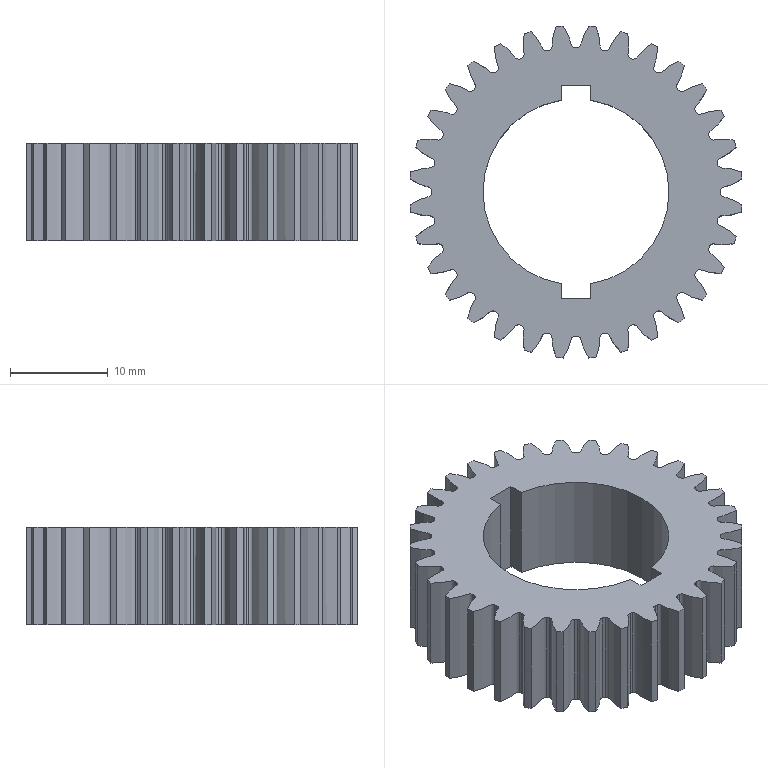Part | SolidWorks | features ICE 3, CirPattern 1, Extrusion 1, RefAxis 1 | 1 solid | 139 faces | box 33.901 x 33.901 x 10 mm | volume 5034 mm3 | cylinder 67 | spline 64 | plane 8 | commonest cylinder face diameters 29.5 x32 34 x32 19 x3